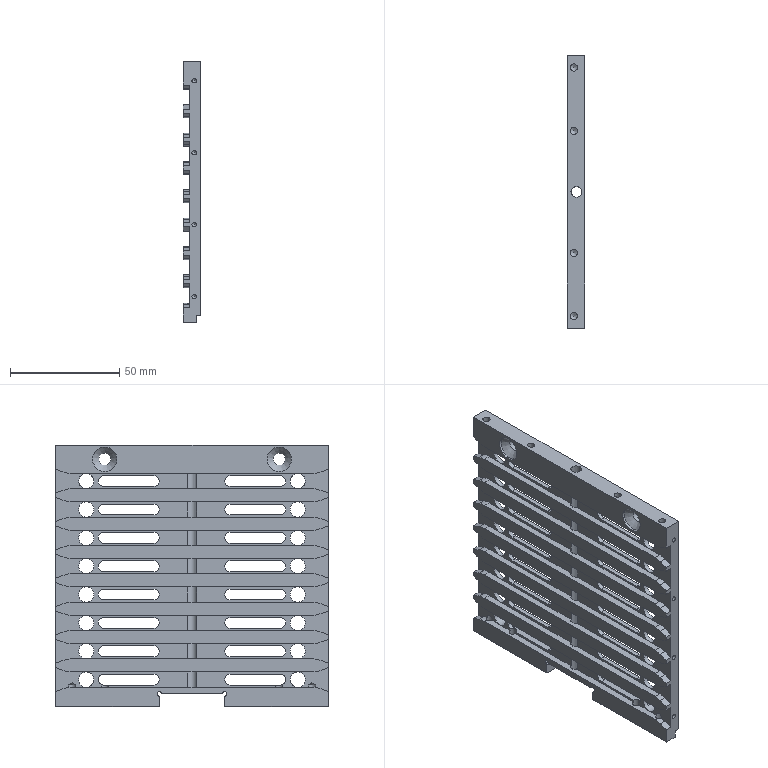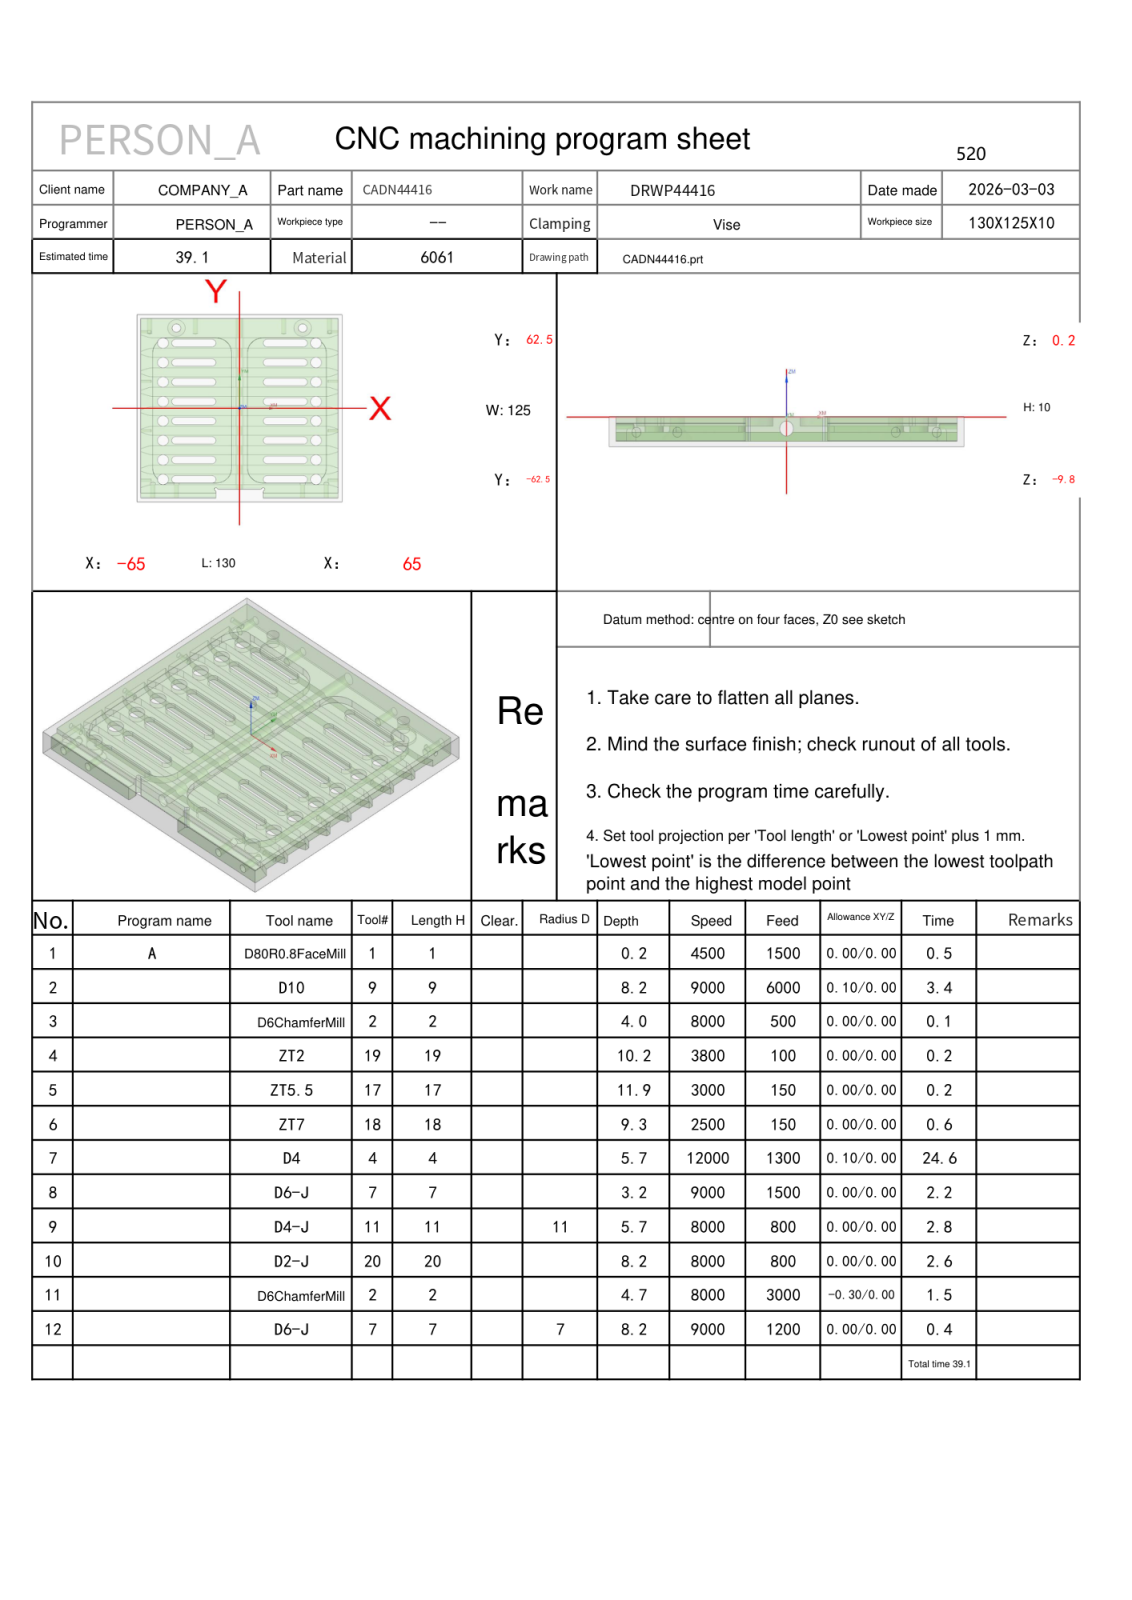NC program | NX | posted by the shop | part box 8 x 125 x 120 mm
Lines 6258 to 7312 of 11100:
N10 T20 M06
(D2-J  D=2. R=0. H=20 ce=0.00 di=0.00)
G00 G90 G54 X13.804 Y-56.738 M03 S8000
G43 H20 Z30.
M08
Z.1
G01 X13.806 Y-56.737 Z.07 F800.
X13.813 Y-56.734 Z.042
X13.824 Y-56.729 Z.018
X13.838 Y-56.721 Z-.004
X13.855 Y-56.712 Z-.023
X13.873 Y-56.7 Z-.04
X13.892 Y-56.687 Z-.054
X13.912 Y-56.671 Z-.066
X13.931 Y-56.653 Z-.076
X13.949 Y-56.633 Z-.084
X13.966 Y-56.611 Z-.09
X13.98 Y-56.586 Z-.095
X13.99 Y-56.56 Z-.098
X13.997 Y-56.531 Z-.099
X14. Y-56.5 Z-.1
Y-55.732
G02 X14.268 Y-54.732 I2. J0.0
X13.268 Y-55. I-1. J1.732
G01 X10.72
X10.704 Y-55.01
X10.719 Y-55.04 Z-.102
X10.762 Y-55.086 Z-.104
X10.83 Y-55.146 Z-.106
X10.921 Y-55.218 Z-.11
X11.169 Y-55.392 Z-.118
X11.442 Y-55.567 Z-.127
X11.799 Y-55.769 Z-.138
X12.179 Y-55.959 Z-.15
X12.572 Y-56.133 Z-.162
X12.968 Y-56.287 Z-.173
X13.298 Y-56.397 Z-.182
X13.615 Y-56.487 Z-.19
X13.743 Y-56.515 Z-.194
X13.849 Y-56.531 Z-.196
X13.93 Y-56.535 Z-.198
X13.982 Y-56.525 Z-.2
X14. Y-56.5
Y-55.732
G02 X14.268 Y-54.732 I2. J0.0
X13.268 Y-55. I-1. J1.732
G01 X10.72
X10.704 Y-55.01
X10.719 Y-55.04 Z-.202
X10.762 Y-55.086 Z-.204
X10.83 Y-55.146 Z-.206
X10.921 Y-55.218 Z-.21
X11.169 Y-55.392 Z-.218
X11.442 Y-55.567 Z-.227
X11.799 Y-55.769 Z-.238
X12.179 Y-55.959 Z-.25
X12.572 Y-56.133 Z-.262
X12.968 Y-56.287 Z-.273
X13.298 Y-56.397 Z-.282
X13.615 Y-56.487 Z-.29
X13.743 Y-56.515 Z-.294
X13.849 Y-56.531 Z-.296
X13.93 Y-56.535 Z-.298
X13.982 Y-56.525 Z-.3
X14. Y-56.5
Y-55.732
G02 X14.268 Y-54.732 I2. J0.0
X13.268 Y-55. I-1. J1.732
G01 X10.72
X10.704 Y-55.01
X10.719 Y-55.04 Z-.302
X10.762 Y-55.086 Z-.304
X10.83 Y-55.146 Z-.306
X10.921 Y-55.218 Z-.31
X11.169 Y-55.392 Z-.318
X11.442 Y-55.567 Z-.327
X11.799 Y-55.769 Z-.338
X12.179 Y-55.959 Z-.35
X12.572 Y-56.133 Z-.362
X12.968 Y-56.287 Z-.373
X13.298 Y-56.397 Z-.382
X13.615 Y-56.487 Z-.39
X13.743 Y-56.515 Z-.394
X13.849 Y-56.531 Z-.396
X13.93 Y-56.535 Z-.398
X13.982 Y-56.525 Z-.4
X14. Y-56.5
Y-55.732
G02 X14.268 Y-54.732 I2. J0.0
X13.268 Y-55. I-1. J1.732
G01 X10.72
X10.704 Y-55.01
X10.719 Y-55.04 Z-.402
X10.762 Y-55.086 Z-.404
X10.83 Y-55.146 Z-.406
X10.921 Y-55.218 Z-.41
X11.169 Y-55.392 Z-.418
X11.442 Y-55.567 Z-.427
X11.799 Y-55.769 Z-.438
X12.179 Y-55.959 Z-.45
X12.572 Y-56.133 Z-.462
X12.968 Y-56.287 Z-.473
X13.298 Y-56.397 Z-.482
X13.615 Y-56.487 Z-.49
X13.743 Y-56.515 Z-.494
X13.849 Y-56.531 Z-.496
X13.93 Y-56.535 Z-.498
X13.982 Y-56.525 Z-.5
X14. Y-56.5
Y-55.732
G02 X14.268 Y-54.732 I2. J0.0
X13.268 Y-55. I-1. J1.732
G01 X10.72
X10.704 Y-55.01
X10.719 Y-55.04 Z-.502
X10.762 Y-55.086 Z-.504
X10.83 Y-55.146 Z-.506
X10.921 Y-55.218 Z-.51
X11.169 Y-55.392 Z-.518
X11.442 Y-55.567 Z-.527
X11.799 Y-55.769 Z-.538
X12.179 Y-55.959 Z-.55
X12.572 Y-56.133 Z-.562
X12.968 Y-56.287 Z-.573
X13.298 Y-56.397 Z-.582
X13.615 Y-56.487 Z-.59
X13.743 Y-56.515 Z-.594
X13.849 Y-56.531 Z-.596
X13.93 Y-56.535 Z-.598
X13.982 Y-56.525 Z-.6
X14. Y-56.5
Y-55.732
G02 X14.268 Y-54.732 I2. J0.0
X13.268 Y-55. I-1. J1.732
G01 X10.72
X10.704 Y-55.01
X10.719 Y-55.04 Z-.602
X10.762 Y-55.086 Z-.604
X10.83 Y-55.146 Z-.606
X10.921 Y-55.218 Z-.61
X11.169 Y-55.392 Z-.618
X11.442 Y-55.567 Z-.627
X11.799 Y-55.769 Z-.638
X12.179 Y-55.959 Z-.65
X12.572 Y-56.133 Z-.662
X12.968 Y-56.287 Z-.673
X13.298 Y-56.397 Z-.682
X13.615 Y-56.487 Z-.69
X13.743 Y-56.515 Z-.694
X13.849 Y-56.531 Z-.696
X13.93 Y-56.535 Z-.698
X13.982 Y-56.525 Z-.7
X14. Y-56.5
Y-55.732
G02 X14.268 Y-54.732 I2. J0.0
X13.268 Y-55. I-1. J1.732
G01 X10.72
X10.704 Y-55.01
X10.719 Y-55.04 Z-.702
X10.762 Y-55.086 Z-.704
X10.83 Y-55.146 Z-.706
X10.921 Y-55.218 Z-.71
X11.169 Y-55.392 Z-.718
X11.442 Y-55.567 Z-.727
X11.799 Y-55.769 Z-.738
X12.179 Y-55.959 Z-.75
X12.572 Y-56.133 Z-.762
X12.968 Y-56.287 Z-.773
X13.298 Y-56.397 Z-.782
X13.615 Y-56.487 Z-.79
X13.743 Y-56.515 Z-.794
X13.849 Y-56.531 Z-.796
X13.93 Y-56.535 Z-.798
X13.982 Y-56.525 Z-.8
X14. Y-56.5
Y-55.732
G02 X14.268 Y-54.732 I2. J0.0
X13.268 Y-55. I-1. J1.732
G01 X10.72
X10.704 Y-55.01
X10.719 Y-55.04 Z-.802
X10.762 Y-55.086 Z-.804
X10.83 Y-55.146 Z-.806
X10.921 Y-55.218 Z-.81
X11.169 Y-55.392 Z-.818
X11.442 Y-55.567 Z-.827
X11.799 Y-55.769 Z-.838
X12.179 Y-55.959 Z-.85
X12.572 Y-56.133 Z-.862
X12.968 Y-56.287 Z-.873
X13.298 Y-56.397 Z-.882
X13.615 Y-56.487 Z-.89
X13.743 Y-56.515 Z-.894
X13.849 Y-56.531 Z-.896
X13.93 Y-56.535 Z-.898
X13.982 Y-56.525 Z-.9
X14. Y-56.5
Y-55.732
G02 X14.268 Y-54.732 I2. J0.0
X13.268 Y-55. I-1. J1.732
G01 X10.72
X10.704 Y-55.01
X10.719 Y-55.04 Z-.902
X10.762 Y-55.086 Z-.904
X10.83 Y-55.146 Z-.906
X10.921 Y-55.218 Z-.91
X11.169 Y-55.392 Z-.918
X11.442 Y-55.567 Z-.927
X11.799 Y-55.769 Z-.938
X12.179 Y-55.959 Z-.95
X12.572 Y-56.133 Z-.962
X12.968 Y-56.287 Z-.973
X13.298 Y-56.397 Z-.982
X13.615 Y-56.487 Z-.99
X13.743 Y-56.515 Z-.994
X13.849 Y-56.531 Z-.996
X13.93 Y-56.535 Z-.998
X13.982 Y-56.525 Z-1.
X14. Y-56.5
Y-55.732
G02 X14.268 Y-54.732 I2. J0.0
X13.268 Y-55. I-1. J1.732
G01 X10.72
X10.704 Y-55.01
X10.719 Y-55.04 Z-1.002
X10.762 Y-55.086 Z-1.004
X10.83 Y-55.146 Z-1.006
X10.921 Y-55.218 Z-1.01
X11.169 Y-55.392 Z-1.018
X11.442 Y-55.567 Z-1.027
X11.799 Y-55.769 Z-1.038
X12.179 Y-55.959 Z-1.05
X12.572 Y-56.133 Z-1.062
X12.968 Y-56.287 Z-1.073
X13.298 Y-56.397 Z-1.082
X13.615 Y-56.487 Z-1.09
X13.743 Y-56.515 Z-1.094
X13.849 Y-56.531 Z-1.096
X13.93 Y-56.535 Z-1.098
X13.982 Y-56.525 Z-1.1
X14. Y-56.5
Y-55.732
G02 X14.268 Y-54.732 I2. J0.0
X13.268 Y-55. I-1. J1.732
G01 X10.72
X10.704 Y-55.01
X10.719 Y-55.04 Z-1.102
X10.762 Y-55.086 Z-1.104
X10.83 Y-55.146 Z-1.106
X10.921 Y-55.218 Z-1.11
X11.169 Y-55.392 Z-1.118
X11.442 Y-55.567 Z-1.127
X11.799 Y-55.769 Z-1.138
X12.179 Y-55.959 Z-1.15
X12.572 Y-56.133 Z-1.162
X12.968 Y-56.287 Z-1.173
X13.298 Y-56.397 Z-1.182
X13.615 Y-56.487 Z-1.19
X13.743 Y-56.515 Z-1.194
X13.849 Y-56.531 Z-1.196
X13.93 Y-56.535 Z-1.198
X13.982 Y-56.525 Z-1.2
X14. Y-56.5
Y-55.732
G02 X14.268 Y-54.732 I2. J0.0
X13.268 Y-55. I-1. J1.732
G01 X10.72
X10.704 Y-55.01
X10.719 Y-55.04 Z-1.202
X10.762 Y-55.086 Z-1.204
X10.83 Y-55.146 Z-1.206
X10.921 Y-55.218 Z-1.21
X11.169 Y-55.392 Z-1.218
X11.442 Y-55.567 Z-1.227
X11.799 Y-55.769 Z-1.238
X12.179 Y-55.959 Z-1.25
X12.572 Y-56.133 Z-1.262
X12.968 Y-56.287 Z-1.273
X13.298 Y-56.397 Z-1.282
X13.615 Y-56.487 Z-1.29
X13.743 Y-56.515 Z-1.294
X13.849 Y-56.531 Z-1.296
X13.93 Y-56.535 Z-1.298
X13.982 Y-56.525 Z-1.3
X14. Y-56.5
Y-55.732
G02 X14.268 Y-54.732 I2. J0.0
X13.268 Y-55. I-1. J1.732
G01 X10.72
X10.704 Y-55.01
X10.719 Y-55.04 Z-1.302
X10.762 Y-55.086 Z-1.304
X10.83 Y-55.146 Z-1.306
X10.921 Y-55.218 Z-1.31
X11.169 Y-55.392 Z-1.318
X11.442 Y-55.567 Z-1.327
X11.799 Y-55.769 Z-1.338
X12.179 Y-55.959 Z-1.35
X12.572 Y-56.133 Z-1.362
X12.968 Y-56.287 Z-1.373
X13.298 Y-56.397 Z-1.382
X13.615 Y-56.487 Z-1.39
X13.743 Y-56.515 Z-1.394
X13.849 Y-56.531 Z-1.396
X13.93 Y-56.535 Z-1.398
X13.982 Y-56.525 Z-1.4
X14. Y-56.5
Y-55.732
G02 X14.268 Y-54.732 I2. J0.0
X13.268 Y-55. I-1. J1.732
G01 X10.72
X10.704 Y-55.01
X10.719 Y-55.04 Z-1.402
X10.762 Y-55.086 Z-1.404
X10.83 Y-55.146 Z-1.406
X10.921 Y-55.218 Z-1.41
X11.169 Y-55.392 Z-1.418
X11.442 Y-55.567 Z-1.427
X11.799 Y-55.769 Z-1.438
X12.179 Y-55.959 Z-1.45
X12.572 Y-56.133 Z-1.462
X12.968 Y-56.287 Z-1.473
X13.298 Y-56.397 Z-1.482
X13.615 Y-56.487 Z-1.49
X13.743 Y-56.515 Z-1.494
X13.849 Y-56.531 Z-1.496
X13.93 Y-56.535 Z-1.498
X13.982 Y-56.525 Z-1.5
X14. Y-56.5
Y-55.732
G02 X14.268 Y-54.732 I2. J0.0
X13.268 Y-55. I-1. J1.732
G01 X10.72
X10.704 Y-55.01
X10.719 Y-55.04 Z-1.502
X10.762 Y-55.086 Z-1.504
X10.83 Y-55.146 Z-1.506
X10.921 Y-55.218 Z-1.51
X11.169 Y-55.392 Z-1.518
X11.442 Y-55.567 Z-1.527
X11.799 Y-55.769 Z-1.538
X12.179 Y-55.959 Z-1.55
X12.572 Y-56.133 Z-1.562
X12.968 Y-56.287 Z-1.573
X13.298 Y-56.397 Z-1.582
X13.615 Y-56.487 Z-1.59
X13.743 Y-56.515 Z-1.594
X13.849 Y-56.531 Z-1.596
X13.93 Y-56.535 Z-1.598
X13.982 Y-56.525 Z-1.6
X14. Y-56.5
Y-55.732
G02 X14.268 Y-54.732 I2. J0.0
X13.268 Y-55. I-1. J1.732
G01 X10.72
X10.704 Y-55.01
X10.719 Y-55.04 Z-1.602
X10.762 Y-55.086 Z-1.604
X10.83 Y-55.146 Z-1.606
X10.921 Y-55.218 Z-1.61
X11.169 Y-55.392 Z-1.618
X11.442 Y-55.567 Z-1.627
X11.799 Y-55.769 Z-1.638
X12.179 Y-55.959 Z-1.65
X12.572 Y-56.133 Z-1.662
X12.968 Y-56.287 Z-1.673
X13.298 Y-56.397 Z-1.682
X13.615 Y-56.487 Z-1.69
X13.743 Y-56.515 Z-1.694
X13.849 Y-56.531 Z-1.696
X13.93 Y-56.535 Z-1.698
X13.982 Y-56.525 Z-1.7
X14. Y-56.5
Y-55.732
G02 X14.268 Y-54.732 I2. J0.0
X13.268 Y-55. I-1. J1.732
G01 X10.72
X10.704 Y-55.01
X10.719 Y-55.04 Z-1.702
X10.762 Y-55.086 Z-1.704
X10.83 Y-55.146 Z-1.706
X10.921 Y-55.218 Z-1.71
X11.169 Y-55.392 Z-1.718
X11.442 Y-55.567 Z-1.727
X11.799 Y-55.769 Z-1.738
X12.179 Y-55.959 Z-1.75
X12.572 Y-56.133 Z-1.762
X12.968 Y-56.287 Z-1.773
X13.298 Y-56.397 Z-1.782
X13.615 Y-56.487 Z-1.79
X13.743 Y-56.515 Z-1.794
X13.849 Y-56.531 Z-1.796
X13.93 Y-56.535 Z-1.798
X13.982 Y-56.525 Z-1.8
X14. Y-56.5
Y-55.732
G02 X14.268 Y-54.732 I2. J0.0
X13.268 Y-55. I-1. J1.732
G01 X10.72
X10.704 Y-55.01
X10.719 Y-55.04 Z-1.802
X10.762 Y-55.086 Z-1.804
X10.83 Y-55.146 Z-1.806
X10.921 Y-55.218 Z-1.81
X11.169 Y-55.392 Z-1.818
X11.442 Y-55.567 Z-1.827
X11.799 Y-55.769 Z-1.838
X12.179 Y-55.959 Z-1.85
X12.572 Y-56.133 Z-1.862
X12.968 Y-56.287 Z-1.873
X13.298 Y-56.397 Z-1.882
X13.615 Y-56.487 Z-1.89
X13.743 Y-56.515 Z-1.894
X13.849 Y-56.531 Z-1.896
X13.93 Y-56.535 Z-1.898
X13.982 Y-56.525 Z-1.9
X14. Y-56.5
Y-55.732
G02 X14.268 Y-54.732 I2. J0.0
X13.268 Y-55. I-1. J1.732
G01 X10.72
X10.704 Y-55.01
X10.719 Y-55.04 Z-1.902
X10.762 Y-55.086 Z-1.904
X10.83 Y-55.146 Z-1.906
X10.921 Y-55.218 Z-1.91
X11.169 Y-55.392 Z-1.918
X11.442 Y-55.567 Z-1.927
X11.799 Y-55.769 Z-1.938
X12.179 Y-55.959 Z-1.95
X12.572 Y-56.133 Z-1.962
X12.968 Y-56.287 Z-1.973
X13.298 Y-56.397 Z-1.982
X13.615 Y-56.487 Z-1.99
X13.743 Y-56.515 Z-1.994
X13.849 Y-56.531 Z-1.996
X13.93 Y-56.535 Z-1.998
X13.982 Y-56.525 Z-2.
X14. Y-56.5
Y-55.732
G02 X14.268 Y-54.732 I2. J0.0
X13.268 Y-55. I-1. J1.732
G01 X10.72
X10.704 Y-55.014
X10.71 Y-55.056 Z-2.001
X10.735 Y-55.121 Z-2.003
X10.778 Y-55.209 Z-2.004
X10.953 Y-55.503 Z-2.011
X11.191 Y-55.863 Z-2.019
X11.365 Y-56.109 Z-2.025
X11.56 Y-56.373 Z-2.031
X11.789 Y-56.672 Z-2.038
X12.046 Y-56.993 Z-2.046
X12.317 Y-57.32 Z-2.054
X12.585 Y-57.63 Z-2.062
X12.835 Y-57.908 Z-2.069
X13.057 Y-58.145 Z-2.075
X13.265 Y-58.356 Z-2.081
X13.571 Y-58.648 Z-2.089
X13.822 Y-58.864 Z-2.096
X13.897 Y-58.919 Z-2.097
X13.953 Y-58.953 Z-2.099
X13.988 Y-58.964 Z-2.1
X14. Y-58.95
Y-55.732
G02 X14.268 Y-54.732 I2. J0.0
X13.268 Y-55. I-1. J1.732
G01 X10.051
X10.037 Y-55.014
X10.048 Y-55.056 Z-2.101
X10.082 Y-55.121 Z-2.103
X10.138 Y-55.209 Z-2.104
X10.405 Y-55.566 Z-2.112
X10.661 Y-55.878 Z-2.119
X10.861 Y-56.111 Z-2.125
X11.098 Y-56.375 Z-2.131
X11.376 Y-56.674 Z-2.138
X11.685 Y-56.995 Z-2.146
X12.011 Y-57.322 Z-2.154
X12.332 Y-57.632 Z-2.162
X12.63 Y-57.909 Z-2.169
X12.893 Y-58.146 Z-2.175
X13.125 Y-58.346 Z-2.181
X13.437 Y-58.599 Z-2.188
X13.792 Y-58.864 Z-2.196
X13.879 Y-58.919 Z-2.197
X13.945 Y-58.953 Z-2.199
X13.986 Y-58.964 Z-2.2
X14. Y-58.95
Y-55.732
G02 X14.268 Y-54.732 I2. J0.0
X13.268 Y-55. I-1. J1.732
G01 X10.051
X10.037 Y-55.014
X10.048 Y-55.056 Z-2.201
X10.082 Y-55.121 Z-2.203
X10.138 Y-55.209 Z-2.204
X10.405 Y-55.566 Z-2.212
X10.66 Y-55.879 Z-2.219
X10.861 Y-56.112 Z-2.225
X11.098 Y-56.377 Z-2.231
X11.375 Y-56.676 Z-2.238
X11.685 Y-56.998 Z-2.246
X12.01 Y-57.324 Z-2.254
X12.331 Y-57.634 Z-2.262
X12.629 Y-57.912 Z-2.269
X12.893 Y-58.148 Z-2.275
X13.125 Y-58.348 Z-2.281
X13.436 Y-58.601 Z-2.288
X13.792 Y-58.865 Z-2.296
X13.879 Y-58.919 Z-2.297
X13.945 Y-58.953 Z-2.299
X13.986 Y-58.964 Z-2.3
X14. Y-58.95
Y-55.732
G02 X14.268 Y-54.732 I2. J0.0
X13.268 Y-55. I-1. J1.732
G01 X10.051
X10.037 Y-55.014
X10.048 Y-55.056 Z-2.301
X10.082 Y-55.121 Z-2.303
X10.138 Y-55.209 Z-2.304
X10.405 Y-55.566 Z-2.312
X10.66 Y-55.879 Z-2.319
X10.861 Y-56.112 Z-2.325
X11.098 Y-56.377 Z-2.331
X11.375 Y-56.676 Z-2.338
X11.685 Y-56.998 Z-2.346
X12.01 Y-57.324 Z-2.354
X12.331 Y-57.634 Z-2.362
X12.629 Y-57.912 Z-2.369
X12.893 Y-58.148 Z-2.375
X13.125 Y-58.348 Z-2.381
X13.436 Y-58.601 Z-2.388
X13.792 Y-58.865 Z-2.396
X13.879 Y-58.919 Z-2.397
X13.945 Y-58.953 Z-2.399
X13.986 Y-58.964 Z-2.4
X14. Y-58.95
Y-55.732
G02 X14.268 Y-54.732 I2. J0.0
X13.268 Y-55. I-1. J1.732
G01 X10.051
X10.037 Y-55.014
X10.048 Y-55.056 Z-2.401
X10.082 Y-55.121 Z-2.403
X10.138 Y-55.209 Z-2.404
X10.405 Y-55.566 Z-2.412
X10.66 Y-55.879 Z-2.419
X10.861 Y-56.112 Z-2.425
X11.098 Y-56.377 Z-2.431
X11.375 Y-56.676 Z-2.438
X11.685 Y-56.998 Z-2.446
X12.01 Y-57.324 Z-2.454
X12.331 Y-57.634 Z-2.462
X12.629 Y-57.912 Z-2.469
X12.893 Y-58.148 Z-2.475
X13.125 Y-58.348 Z-2.481
X13.436 Y-58.601 Z-2.488
X13.792 Y-58.865 Z-2.496
X13.879 Y-58.919 Z-2.497
X13.945 Y-58.953 Z-2.499
X13.986 Y-58.964 Z-2.5
X14. Y-58.95
Y-55.732
G02 X14.268 Y-54.732 I2. J0.0
X13.268 Y-55. I-1. J1.732
G01 X10.051
X10.037 Y-55.014
X10.048 Y-55.056 Z-2.501
X10.082 Y-55.121 Z-2.503
X10.138 Y-55.209 Z-2.504
X10.405 Y-55.566 Z-2.512
X10.66 Y-55.879 Z-2.519
X10.861 Y-56.112 Z-2.525
X11.098 Y-56.377 Z-2.531
X11.375 Y-56.676 Z-2.538
X11.685 Y-56.998 Z-2.546
X12.01 Y-57.324 Z-2.554
X12.331 Y-57.634 Z-2.562
X12.629 Y-57.912 Z-2.569
X12.893 Y-58.148 Z-2.575
X13.125 Y-58.348 Z-2.581
X13.436 Y-58.601 Z-2.588
X13.792 Y-58.865 Z-2.596
X13.879 Y-58.919 Z-2.597
X13.945 Y-58.953 Z-2.599
X13.986 Y-58.964 Z-2.6
X14. Y-58.95
Y-55.732
G02 X14.268 Y-54.732 I2. J0.0
X13.268 Y-55. I-1. J1.732
G01 X10.051
X10.037 Y-55.014
X10.048 Y-55.056 Z-2.601
X10.082 Y-55.121 Z-2.603
X10.138 Y-55.209 Z-2.604
X10.405 Y-55.566 Z-2.612
X10.66 Y-55.879 Z-2.619
X10.861 Y-56.112 Z-2.625
X11.098 Y-56.377 Z-2.631
X11.375 Y-56.676 Z-2.638
X11.685 Y-56.998 Z-2.646
X12.01 Y-57.324 Z-2.654
X12.331 Y-57.634 Z-2.662
X12.629 Y-57.912 Z-2.669
X12.893 Y-58.148 Z-2.675
X13.125 Y-58.348 Z-2.681
X13.436 Y-58.601 Z-2.688
X13.792 Y-58.865 Z-2.696
X13.879 Y-58.919 Z-2.697
X13.945 Y-58.953 Z-2.699
X13.986 Y-58.964 Z-2.7
X14. Y-58.95
Y-55.732
G02 X14.268 Y-54.732 I2. J0.0
X13.268 Y-55. I-1. J1.732
G01 X10.051
X10.037 Y-55.014
X10.048 Y-55.056 Z-2.701
X10.082 Y-55.121 Z-2.703
X10.138 Y-55.209 Z-2.704
X10.405 Y-55.566 Z-2.712
X10.66 Y-55.879 Z-2.719
X10.861 Y-56.112 Z-2.725
X11.098 Y-56.377 Z-2.731
X11.375 Y-56.676 Z-2.738
X11.685 Y-56.998 Z-2.746
X12.01 Y-57.324 Z-2.754
X12.331 Y-57.634 Z-2.762
X12.629 Y-57.912 Z-2.769
X12.893 Y-58.148 Z-2.775
X13.125 Y-58.348 Z-2.781
X13.436 Y-58.601 Z-2.788
X13.792 Y-58.865 Z-2.796
X13.879 Y-58.919 Z-2.797
X13.945 Y-58.953 Z-2.799
X13.986 Y-58.964 Z-2.8
X14. Y-58.95
Y-55.732
G02 X14.268 Y-54.732 I2. J0.0
X13.268 Y-55. I-1. J1.732
G01 X10.051
X10.037 Y-55.014
X10.048 Y-55.056 Z-2.801
X10.082 Y-55.121 Z-2.803
X10.138 Y-55.209 Z-2.804
X10.405 Y-55.566 Z-2.812
X10.66 Y-55.879 Z-2.819
X10.861 Y-56.112 Z-2.825
X11.098 Y-56.377 Z-2.831
X11.375 Y-56.676 Z-2.838
X11.685 Y-56.998 Z-2.846
X12.01 Y-57.324 Z-2.854
X12.331 Y-57.634 Z-2.862
X12.629 Y-57.912 Z-2.869
X12.893 Y-58.148 Z-2.875
X13.125 Y-58.348 Z-2.881
X13.436 Y-58.601 Z-2.888
X13.792 Y-58.865 Z-2.896
X13.879 Y-58.919 Z-2.897
X13.945 Y-58.953 Z-2.899
X13.986 Y-58.964 Z-2.9
X14. Y-58.95
Y-55.732
G02 X14.268 Y-54.732 I2. J0.0
X13.268 Y-55. I-1. J1.732
G01 X10.051
X10.037 Y-55.014
X10.048 Y-55.056 Z-2.901
X10.082 Y-55.121 Z-2.903
X10.138 Y-55.209 Z-2.904
X10.405 Y-55.566 Z-2.912
X10.66 Y-55.879 Z-2.919
X10.861 Y-56.112 Z-2.925
X11.098 Y-56.377 Z-2.931
X11.375 Y-56.676 Z-2.938
X11.685 Y-56.998 Z-2.946
X12.01 Y-57.324 Z-2.954
X12.331 Y-57.634 Z-2.962
X12.629 Y-57.912 Z-2.969
X12.893 Y-58.148 Z-2.975
X13.125 Y-58.348 Z-2.981
X13.436 Y-58.601 Z-2.988
X13.792 Y-58.865 Z-2.996
X13.879 Y-58.919 Z-2.997
X13.945 Y-58.953 Z-2.999
X13.986 Y-58.964 Z-3.
X14. Y-58.95
Y-55.732
G02 X14.268 Y-54.732 I2. J0.0
X13.268 Y-55. I-1. J1.732
G01 X10.051
X10.037 Y-55.014
X10.048 Y-55.056 Z-3.001
X10.082 Y-55.121 Z-3.003
X10.138 Y-55.209 Z-3.004
X10.405 Y-55.566 Z-3.012
X10.66 Y-55.879 Z-3.019
X10.861 Y-56.112 Z-3.025
X11.098 Y-56.377 Z-3.031
X11.375 Y-56.676 Z-3.038
X11.685 Y-56.998 Z-3.046
X12.01 Y-57.324 Z-3.054
X12.331 Y-57.634 Z-3.062
X12.629 Y-57.912 Z-3.069
X12.893 Y-58.148 Z-3.075
X13.125 Y-58.348 Z-3.081
X13.436 Y-58.601 Z-3.088
X13.792 Y-58.865 Z-3.096
X13.879 Y-58.919 Z-3.097
X13.945 Y-58.953 Z-3.099
X13.986 Y-58.964 Z-3.1
X14. Y-58.95
Y-55.732
G02 X14.268 Y-54.732 I2. J0.0
X13.268 Y-55. I-1. J1.732
G01 X10.051
X10.037 Y-55.014
X10.048 Y-55.056 Z-3.101
X10.082 Y-55.121 Z-3.103
X10.138 Y-55.209 Z-3.104
X10.405 Y-55.566 Z-3.112
X10.66 Y-55.879 Z-3.119
X10.861 Y-56.112 Z-3.125
X11.098 Y-56.377 Z-3.131
X11.375 Y-56.676 Z-3.138
X11.685 Y-56.998 Z-3.146
X12.01 Y-57.324 Z-3.154
X12.331 Y-57.634 Z-3.162
X12.629 Y-57.912 Z-3.169
X12.893 Y-58.148 Z-3.175
X13.125 Y-58.348 Z-3.181
X13.436 Y-58.601 Z-3.188
X13.792 Y-58.865 Z-3.196
X13.879 Y-58.919 Z-3.197
X13.945 Y-58.953 Z-3.199
X13.986 Y-58.964 Z-3.2
X14. Y-58.95
Y-55.732
G02 X14.268 Y-54.732 I2. J0.0
X13.268 Y-55. I-1. J1.732
G01 X10.051
X10.037 Y-55.014
X10.048 Y-55.056 Z-3.201
X10.082 Y-55.121 Z-3.203
X10.138 Y-55.209 Z-3.204
X10.405 Y-55.566 Z-3.212
X10.66 Y-55.879 Z-3.219
X10.861 Y-56.112 Z-3.225
X11.098 Y-56.377 Z-3.231
X11.375 Y-56.676 Z-3.238
X11.685 Y-56.998 Z-3.246
X12.01 Y-57.324 Z-3.254
X12.331 Y-57.634 Z-3.262
X12.629 Y-57.912 Z-3.269
X12.893 Y-58.148 Z-3.275
X13.125 Y-58.348 Z-3.281
X13.436 Y-58.601 Z-3.288
X13.792 Y-58.865 Z-3.296
X13.879 Y-58.919 Z-3.297
X13.945 Y-58.953 Z-3.299
X13.986 Y-58.964 Z-3.3
X14. Y-58.95
Y-55.732
G02 X14.268 Y-54.732 I2. J0.0
X13.268 Y-55. I-1. J1.732
G01 X10.051
X10.037 Y-55.014
X10.048 Y-55.056 Z-3.301
X10.082 Y-55.121 Z-3.303
X10.138 Y-55.209 Z-3.304
X10.405 Y-55.566 Z-3.312
X10.66 Y-55.879 Z-3.319
X10.861 Y-56.112 Z-3.325
X11.098 Y-56.377 Z-3.331
X11.375 Y-56.676 Z-3.338
X11.685 Y-56.998 Z-3.346
X12.01 Y-57.324 Z-3.354
X12.331 Y-57.634 Z-3.362
X12.629 Y-57.912 Z-3.369
X12.893 Y-58.148 Z-3.375
X13.125 Y-58.348 Z-3.381
X13.436 Y-58.601 Z-3.388
X13.792 Y-58.865 Z-3.396
X13.879 Y-58.919 Z-3.397
X13.945 Y-58.953 Z-3.399
X13.986 Y-58.964 Z-3.4
X14. Y-58.95
Y-55.732
G02 X14.268 Y-54.732 I2. J0.0
X13.268 Y-55. I-1. J1.732
G01 X10.051
X10.037 Y-55.014
X10.048 Y-55.056 Z-3.401
X10.082 Y-55.121 Z-3.403
X10.138 Y-55.209 Z-3.404
X10.405 Y-55.566 Z-3.412
X10.66 Y-55.879 Z-3.419
X10.861 Y-56.112 Z-3.425
X11.098 Y-56.377 Z-3.431
X11.375 Y-56.676 Z-3.438
X11.685 Y-56.998 Z-3.446
X12.01 Y-57.324 Z-3.454
X12.331 Y-57.634 Z-3.462
X12.629 Y-57.912 Z-3.469
X12.893 Y-58.148 Z-3.475
X13.125 Y-58.348 Z-3.481
X13.436 Y-58.601 Z-3.488
X13.792 Y-58.865 Z-3.496
X13.879 Y-58.919 Z-3.497
X13.945 Y-58.953 Z-3.499
X13.986 Y-58.964 Z-3.5
X14. Y-58.95
Y-55.732
G02 X14.268 Y-54.732 I2. J0.0
X13.268 Y-55. I-1. J1.732
G01 X10.051
X10.037 Y-55.014
X10.048 Y-55.056 Z-3.501
X10.082 Y-55.121 Z-3.503
X10.138 Y-55.209 Z-3.504
X10.405 Y-55.566 Z-3.512
X10.66 Y-55.879 Z-3.519
X10.861 Y-56.112 Z-3.525
X11.098 Y-56.377 Z-3.531
X11.375 Y-56.676 Z-3.538
X11.685 Y-56.998 Z-3.546
X12.01 Y-57.324 Z-3.554
X12.331 Y-57.634 Z-3.562
X12.629 Y-57.912 Z-3.569
X12.893 Y-58.148 Z-3.575
X13.125 Y-58.348 Z-3.581
X13.436 Y-58.601 Z-3.588
X13.792 Y-58.865 Z-3.596
X13.879 Y-58.919 Z-3.597
X13.945 Y-58.953 Z-3.599
X13.986 Y-58.964 Z-3.6
X14. Y-58.95
Y-55.732
G02 X14.268 Y-54.732 I2. J0.0
X13.268 Y-55. I-1. J1.732
G01 X10.051
X10.037 Y-55.014
X10.048 Y-55.056 Z-3.601
X10.082 Y-55.121 Z-3.603
X10.138 Y-55.209 Z-3.604
X10.405 Y-55.566 Z-3.612
X10.66 Y-55.879 Z-3.619
X10.861 Y-56.112 Z-3.625
X11.098 Y-56.377 Z-3.631
X11.375 Y-56.676 Z-3.638
X11.685 Y-56.998 Z-3.646
X12.01 Y-57.324 Z-3.654
X12.331 Y-57.634 Z-3.662
X12.629 Y-57.912 Z-3.669
X12.893 Y-58.148 Z-3.675
X13.125 Y-58.348 Z-3.681
X13.436 Y-58.601 Z-3.688
X13.792 Y-58.865 Z-3.696
X13.879 Y-58.919 Z-3.697
X13.945 Y-58.953 Z-3.699
X13.986 Y-58.964 Z-3.7
X14. Y-58.95
Y-55.732
G02 X14.268 Y-54.732 I2. J0.0
X13.268 Y-55. I-1. J1.732
G01 X10.051
X10.037 Y-55.014
X10.048 Y-55.056 Z-3.701
X10.082 Y-55.121 Z-3.703
X10.138 Y-55.209 Z-3.704
X10.405 Y-55.566 Z-3.712
X10.66 Y-55.879 Z-3.719
X10.861 Y-56.112 Z-3.725
X11.098 Y-56.377 Z-3.731
X11.375 Y-56.676 Z-3.738
X11.685 Y-56.998 Z-3.746
X12.01 Y-57.324 Z-3.754
X12.331 Y-57.634 Z-3.762
X12.629 Y-57.912 Z-3.769
X12.893 Y-58.148 Z-3.775
X13.125 Y-58.348 Z-3.781
X13.436 Y-58.601 Z-3.788
X13.792 Y-58.865 Z-3.796
X13.879 Y-58.919 Z-3.797
X13.945 Y-58.953 Z-3.799
X13.986 Y-58.964 Z-3.8
X14. Y-58.95
Y-55.732
G02 X14.268 Y-54.732 I2. J0.0
X13.268 Y-55. I-1. J1.732
G01 X10.051
X10.037 Y-55.014
X10.048 Y-55.056 Z-3.801
X10.082 Y-55.121 Z-3.803
X10.138 Y-55.209 Z-3.804
X10.405 Y-55.566 Z-3.812
X10.66 Y-55.879 Z-3.819
X10.861 Y-56.112 Z-3.825
X11.098 Y-56.377 Z-3.831
X11.375 Y-56.676 Z-3.838
X11.685 Y-56.998 Z-3.846
X12.01 Y-57.324 Z-3.854
X12.331 Y-57.634 Z-3.862
X12.629 Y-57.912 Z-3.869
X12.893 Y-58.148 Z-3.875
X13.125 Y-58.348 Z-3.881
X13.436 Y-58.601 Z-3.888
X13.792 Y-58.865 Z-3.896
X13.879 Y-58.919 Z-3.897
X13.945 Y-58.953 Z-3.899
X13.986 Y-58.964 Z-3.9
X14. Y-58.95
Y-55.732
G02 X14.268 Y-54.732 I2. J0.0
X13.268 Y-55. I-1. J1.732
G01 X10.051
X10.037 Y-55.014
X10.048 Y-55.056 Z-3.901
X10.082 Y-55.121 Z-3.903
X10.138 Y-55.209 Z-3.904
X10.405 Y-55.566 Z-3.912
X10.66 Y-55.879 Z-3.919
X10.861 Y-56.112 Z-3.925
X11.098 Y-56.377 Z-3.931
X11.375 Y-56.676 Z-3.938
X11.685 Y-56.998 Z-3.946
X12.01 Y-57.324 Z-3.954
X12.331 Y-57.634 Z-3.962
X12.629 Y-57.912 Z-3.969
X12.893 Y-58.148 Z-3.975
X13.125 Y-58.348 Z-3.981
X13.436 Y-58.601 Z-3.988
X13.792 Y-58.865 Z-3.996
X13.879 Y-58.919 Z-3.997
X13.945 Y-58.953 Z-3.999
X13.986 Y-58.964 Z-4.
X14. Y-58.95
Y-55.732
G02 X14.268 Y-54.732 I2. J0.0
X13.268 Y-55. I-1. J1.732
G01 X10.051
X10.037 Y-55.014
X10.048 Y-55.056 Z-4.001
X10.082 Y-55.121 Z-4.003
X10.138 Y-55.209 Z-4.004
X10.405 Y-55.566 Z-4.012
X10.66 Y-55.879 Z-4.019
X10.861 Y-56.112 Z-4.025
X11.098 Y-56.377 Z-4.031
X11.375 Y-56.676 Z-4.038
X11.685 Y-56.998 Z-4.046
X12.01 Y-57.324 Z-4.054
X12.331 Y-57.634 Z-4.062
X12.629 Y-57.912 Z-4.069
X12.893 Y-58.148 Z-4.075
X13.125 Y-58.348 Z-4.081
X13.436 Y-58.601 Z-4.088
X13.792 Y-58.865 Z-4.096
X13.879 Y-58.919 Z-4.097
X13.945 Y-58.953 Z-4.099
X13.986 Y-58.964 Z-4.1
X14. Y-58.95
Y-55.732
G02 X14.268 Y-54.732 I2. J0.0
X13.268 Y-55. I-1. J1.732
G01 X10.051
X10.037 Y-55.014
X10.048 Y-55.056 Z-4.101
X10.082 Y-55.121 Z-4.103
X10.138 Y-55.209 Z-4.104
X10.405 Y-55.566 Z-4.112
X10.66 Y-55.879 Z-4.119
X10.861 Y-56.112 Z-4.125
X11.098 Y-56.377 Z-4.131
X11.375 Y-56.676 Z-4.138
X11.685 Y-56.998 Z-4.146
X12.01 Y-57.324 Z-4.154
X12.331 Y-57.634 Z-4.162
X12.629 Y-57.912 Z-4.169
X12.893 Y-58.148 Z-4.175
X13.125 Y-58.348 Z-4.181
X13.436 Y-58.601 Z-4.188
X13.792 Y-58.865 Z-4.196
X13.879 Y-58.919 Z-4.197
X13.945 Y-58.953 Z-4.199
X13.986 Y-58.964 Z-4.2
X14. Y-58.95
Y-55.732
G02 X14.268 Y-54.732 I2. J0.0
X13.268 Y-55. I-1. J1.732
G01 X10.051
X10.037 Y-55.014
X10.048 Y-55.056 Z-4.201
X10.082 Y-55.121 Z-4.203
X10.138 Y-55.209 Z-4.204
X10.405 Y-55.566 Z-4.212
X10.66 Y-55.879 Z-4.219
X10.861 Y-56.112 Z-4.225
X11.098 Y-56.377 Z-4.231
X11.375 Y-56.676 Z-4.238
X11.685 Y-56.998 Z-4.246
X12.01 Y-57.324 Z-4.254
X12.331 Y-57.634 Z-4.262
X12.629 Y-57.912 Z-4.269
X12.893 Y-58.148 Z-4.275
X13.125 Y-58.348 Z-4.281
X13.436 Y-58.601 Z-4.288
X13.792 Y-58.865 Z-4.296
X13.879 Y-58.919 Z-4.297
X13.945 Y-58.953 Z-4.299
X13.986 Y-58.964 Z-4.3
X14. Y-58.95
Y-55.732
G02 X14.268 Y-54.732 I2. J0.0
X13.268 Y-55. I-1. J1.732
G01 X10.051
X10.037 Y-55.014
X10.048 Y-55.056 Z-4.301
X10.082 Y-55.121 Z-4.303
X10.138 Y-55.209 Z-4.304
X10.405 Y-55.566 Z-4.312
X10.66 Y-55.879 Z-4.319
X10.861 Y-56.112 Z-4.325
X11.098 Y-56.377 Z-4.331
X11.375 Y-56.676 Z-4.338
X11.685 Y-56.998 Z-4.346
X12.01 Y-57.324 Z-4.354
X12.331 Y-57.634 Z-4.362
X12.629 Y-57.912 Z-4.369
X12.893 Y-58.148 Z-4.375
X13.125 Y-58.348 Z-4.381
X13.436 Y-58.601 Z-4.388
X13.792 Y-58.865 Z-4.396
X13.879 Y-58.919 Z-4.397
X13.945 Y-58.953 Z-4.399
X13.986 Y-58.964 Z-4.4
X14. Y-58.95
Y-55.732
G02 X14.268 Y-54.732 I2. J0.0
X13.268 Y-55. I-1. J1.732
G01 X10.051
X10.037 Y-55.014
X10.048 Y-55.056 Z-4.401
X10.082 Y-55.121 Z-4.403
X10.138 Y-55.209 Z-4.404
X10.405 Y-55.566 Z-4.412
X10.66 Y-55.879 Z-4.419
X10.861 Y-56.112 Z-4.425
X11.098 Y-56.377 Z-4.431
X11.375 Y-56.676 Z-4.438
X11.685 Y-56.998 Z-4.446
X12.01 Y-57.324 Z-4.454
X12.331 Y-57.634 Z-4.462